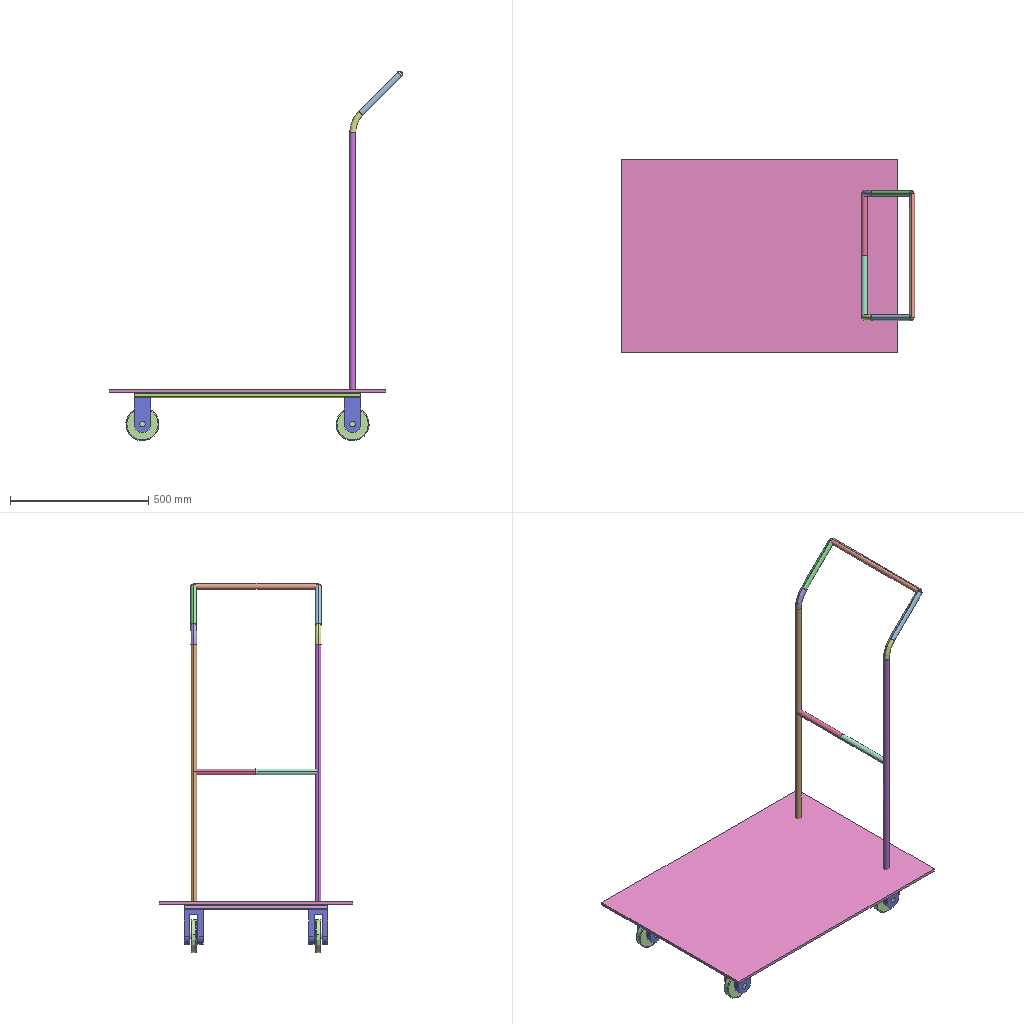Assembly | SolidWorks | 5 different items | 11 placed | box 1061 x 700 x 1336 mm
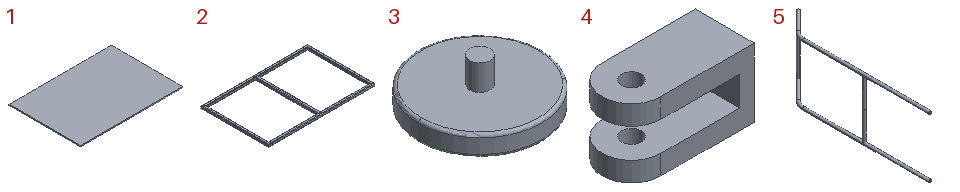Parts list (item | quantity | size | volume | features):
1 | x1 | 1000 x 700 x 10 mm | 7000000 mm3 | features Extrusion 1
2 | x1 | 820 x 520 x 20 mm | 414467 mm3 | features WeldMemberFeat 2, WeldmentFeature 1
3 | x4 | 120 x 120 x 70 mm | 240463 mm3 | features ICE 2, Extrusion 1, Fillet 1
4 | x4 | 125 x 60 x 70 mm | 298982 mm3 | features ICE 2, Extrusion 1, MirrorSolid 1
5 | x1 | 192.011 x 1181 x 471.3 mm | 463241 mm3 | features WeldMemberFeat 3, MirrorSolid 1, WeldmentFeature 1
Mates (type | each side: item.copy, entity, surface, feature):
Concentric | 4.1 face cylinder Cut-Extrude1 | 3.1 face cylinder Boss-Extrude3
Width | 3.1 face plane Boss-Extrude3 | 3.1 face plane Boss-Extrude2 | 4.1 face plane Mirror1 | 4.1 face plane Boss-Extrude1
Coincident | 2.1 face plane Square tube 20 X 20 X 2(1) | 4.1 face plane Mirror1
Coincident | 2.1 face plane Square tube 20 X 20 X 2(1) | 4.1 face plane Boss-Extrude1
Coincident | 2.1 face plane Square tube 20 X 20 X 2(1) | 4.1 face plane Boss-Extrude5
ProfileCenter | 4.1 face plane Boss-Extrude5 | 5.1 face plane Mirror1
Coincident | 2.1 face plane Square tube 20 X 20 X 2(2) | 1.1 face plane Boss-Extrude1
Width | 2.1 face plane Square tube 20 X 20 X 2(1) | 2.1 face plane Square tube 20 X 20 X 2(1) | 1.1 face plane Boss-Extrude1 | 1.1 face plane Boss-Extrude1
Width | 1.1 face plane Boss-Extrude1 | 1.1 face plane Boss-Extrude1 | 2.1 face plane Square tube 20 X 20 X 2(1) | 2.1 face plane Square tube 20 X 20 X 2(1)